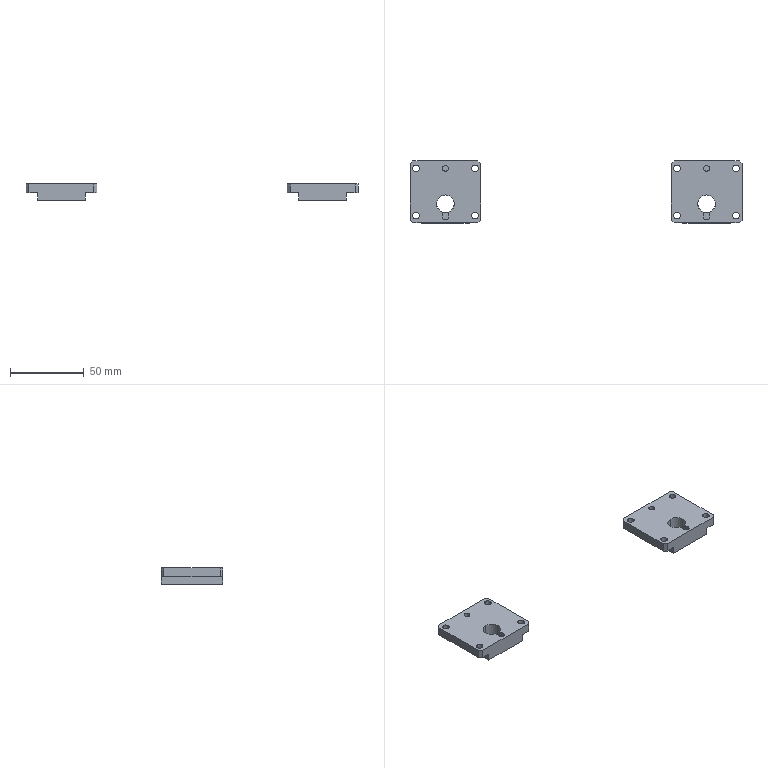NC program | NX | posted with a generic post | part box 225 x 42 x 11 mm
Whole program:
N10 G17 G21 G94 G90
(FLOOR_WALL_COPY , TOOL : D63)
N12 T01 M6
N14 G54
N16 G17 G0 G90 X-58.5 Y0. S6500 M3
N18 G43 Z30. H1
N20 Z3.
N22 G94 G1 Z0. F1500.
N24 X-55.5
N26 X55.5
N28 X58.5
N30 Z3.
N32 G0 Z30.
N34 M5
(DRILLING_COPY_1 , TOOL : D6A45)
N36 T07 M6
N38 G54
N40 G17 G0 G90 X12. Y10. S5000 M3
N42 G43 Z30. H7
N44 G94 G81 G98 Z-1. F250. R3.
N46 X5. Y16.
N48 X-5.
N50 X-12. Y10.
N52 G80
N54 G0 X-12. Y10. Z30.
N56 M5
(DRILLING_COPY_COPY , TOOL : 2.5ZT)
N58 T12 M6
N60 G54
N62 G17 G0 G90 X-12. Y10. S2000 M3
N64 G43 Z30. H12
N66 G94 G83 G98 Z-6.751 F120. Q2. R3.
N68 X-5. Y16. Z-8.251
N70 X5.
N72 X12. Y10. Z-6.751
N74 G80
N76 G0 X12. Y10. Z30.
N78 M5
(FLOOR_WALL_1 , TOOL : D10)
N80 T10 M6
N82 G54
N84 G17 G0 G90 X-31. Y-4.619 S9500 M3
N86 G43 Z30. H10
N88 Z-0.288
N90 G94 G1 X-24.5 Y-0.866 F1000.
N92 G3 X-24. Y0. R1.
N94 G1 Y19. F2500.
N96 X-22. Y21.
N98 X-21.1
N100 Y-21.
N102 X-22.
N104 X-24. Y-19.
N106 Y0.
N108 G3 X-24.5 Y0.866 R1.
N110 G1 X-31. Y4.619
N112 G0 Y-4.619 Z-0.576
N114 G1 X-24.5 Y-0.866 F1000.
N116 G3 X-24. Y0. R1.
N118 G1 Y19. F2500.
N120 X-22. Y21.
N122 X-21.1
N124 Y-21.
N126 X-22.
N128 X-24. Y-19.
N130 Y0.
N132 G3 X-24.5 Y0.866 R1.
N134 G1 X-31. Y4.619
N136 G0 Y-4.619 Z-0.865
N138 G1 X-24.5 Y-0.866 F1000.
N140 G3 X-24. Y0. R1.
N142 G1 Y19. F2500.
N144 X-22. Y21.
N146 X-21.1
N148 Y-21.
N150 X-22.
N152 X-24. Y-19.
N154 Y0.
N156 G3 X-24.5 Y0.866 R1.
N158 G1 X-31. Y4.619
N160 G0 Y-4.619 Z-1.153
N162 G1 X-24.5 Y-0.866 F1000.
N164 G3 X-24. Y0. R1.
N166 G1 Y19. F2500.
N168 X-22. Y21.
N170 X-21.1
N172 Y-21.
N174 X-22.
N176 X-24. Y-19.
N178 Y0.
N180 G3 X-24.5 Y0.866 R1.
N182 G1 X-31. Y4.619
N184 G0 Y-4.619 Z-1.441
N186 G1 X-24.5 Y-0.866 F1000.
N188 G3 X-24. Y0. R1.
N190 G1 Y19. F2500.
N192 X-22. Y21.
N194 X-21.1
N196 Y-21.
N198 X-22.
N200 X-24. Y-19.
N202 Y0.
N204 G3 X-24.5 Y0.866 R1.
N206 G1 X-31. Y4.619
N208 G0 Y-4.619 Z-1.729
N210 G1 X-24.5 Y-0.866 F1000.
N212 G3 X-24. Y0. R1.
N214 G1 Y19. F2500.
N216 X-22. Y21.
N218 X-21.1
N220 Y-21.
N222 X-22.
N224 X-24. Y-19.
N226 Y0.
N228 G3 X-24.5 Y0.866 R1.
N230 G1 X-31. Y4.619
N232 G0 Y-4.619 Z-2.018
N234 G1 X-24.5 Y-0.866 F1000.
N236 G3 X-24. Y0. R1.
N238 G1 Y19. F2500.
N240 X-22. Y21.
N242 X-21.1
N244 Y-21.
N246 X-22.
N248 X-24. Y-19.
N250 Y0.
N252 G3 X-24.5 Y0.866 R1.
N254 G1 X-31. Y4.619
N256 G0 Y-4.619 Z-2.306
N258 G1 X-24.5 Y-0.866 F1000.
N260 G3 X-24. Y0. R1.
N262 G1 Y19. F2500.
N264 X-22. Y21.
N266 X-21.1
N268 Y-21.
N270 X-22.
N272 X-24. Y-19.
N274 Y0.
N276 G3 X-24.5 Y0.866 R1.
N278 G1 X-31. Y4.619
N280 G0 Y-4.619 Z-2.594
N282 G1 X-24.5 Y-0.866 F1000.
N284 G3 X-24. Y0. R1.
N286 G1 Y19. F2500.
N288 X-22. Y21.
N290 X-21.1
N292 Y-21.
N294 X-22.
N296 X-24. Y-19.
N298 Y0.
N300 G3 X-24.5 Y0.866 R1.
N302 G1 X-31. Y4.619
N304 G0 Y-4.619 Z-2.882
N306 G1 X-24.5 Y-0.866 F1000.
N308 G3 X-24. Y0. R1.
N310 G1 Y19. F2500.
N312 X-22. Y21.
N314 X-21.1
N316 Y-21.
N318 X-22.
N320 X-24. Y-19.
N322 Y0.
N324 G3 X-24.5 Y0.866 R1.
N326 G1 X-31. Y4.619
N328 G0 Y-4.619 Z-3.171
N330 G1 X-24.5 Y-0.866 F1000.
N332 G3 X-24. Y0. R1.
N334 G1 Y19. F2500.
N336 X-22. Y21.
N338 X-21.1
N340 Y-21.
N342 X-22.
N344 X-24. Y-19.
N346 Y0.
N348 G3 X-24.5 Y0.866 R1.
N350 G1 X-31. Y4.619
N352 G0 Y-4.619 Z-3.459
N354 G1 X-24.5 Y-0.866 F1000.
N356 G3 X-24. Y0. R1.
N358 G1 Y19. F2500.
N360 X-22. Y21.
N362 X-21.1
N364 Y-21.
N366 X-22.
N368 X-24. Y-19.
N370 Y0.
N372 G3 X-24.5 Y0.866 R1.
N374 G1 X-31. Y4.619
N376 G0 Y-4.619 Z-3.747
N378 G1 X-24.5 Y-0.866 F1000.
N380 G3 X-24. Y0. R1.
N382 G1 Y19. F2500.
N384 X-22. Y21.
N386 X-21.1
N388 Y-21.
N390 X-22.
N392 X-24. Y-19.
N394 Y0.
N396 G3 X-24.5 Y0.866 R1.
N398 G1 X-31. Y4.619
N400 G0 Y-4.619 Z-4.035
N402 G1 X-24.5 Y-0.866 F1000.
N404 G3 X-24. Y0. R1.
N406 G1 Y19. F2500.
N408 X-22. Y21.
N410 X-21.1
N412 Y-21.
N414 X-22.
N416 X-24. Y-19.
N418 Y0.
N420 G3 X-24.5 Y0.866 R1.
N422 G1 X-31. Y4.619
N424 G0 Y-4.619 Z-4.324
N426 G1 X-24.5 Y-0.866 F1000.
N428 G3 X-24. Y0. R1.
N430 G1 Y19. F2500.
N432 X-22. Y21.
N434 X-21.1
N436 Y-21.
N438 X-22.
N440 X-24. Y-19.
N442 Y0.
N444 G3 X-24.5 Y0.866 R1.
N446 G1 X-31. Y4.619
N448 G0 Y-4.619 Z-4.612
N450 G1 X-24.5 Y-0.866 F1000.
N452 G3 X-24. Y0. R1.
N454 G1 Y19. F2500.
N456 X-22. Y21.
N458 X-21.1
N460 Y-21.
N462 X-22.
N464 X-24. Y-19.
N466 Y0.
N468 G3 X-24.5 Y0.866 R1.
N470 G1 X-31. Y4.619
N472 G0 Y-4.619 Z-4.9
N474 G1 X-24.5 Y-0.866 F1000.
N476 G3 X-24. Y0. R1.
N478 G1 Y19. F2500.
N480 X-22. Y21.
N482 X-21.1
N484 Y-21.
N486 X-22.
N488 X-24. Y-19.
N490 Y0.
N492 G3 X-24.5 Y0.866 R1.
N494 G1 X-31. Y4.619
N496 G0 Z30.
N498 X31.
N500 Z-0.288
N502 G1 X24.5 Y0.866 F1000.
N504 G3 X24. Y0. R1.
N506 G1 Y-19. F2500.
N508 X22. Y-21.
N510 X21.1
N512 Y21.
N514 X22.
N516 X24. Y19.
N518 Y0.
N520 G3 X24.5 Y-0.866 R1.
N522 G1 X31. Y-4.619
N524 G0 Y4.619 Z-0.576
N526 G1 X24.5 Y0.866 F1000.
N528 G3 X24. Y0. R1.
N530 G1 Y-19. F2500.
N532 X22. Y-21.
N534 X21.1
N536 Y21.
N538 X22.
N540 X24. Y19.
N542 Y0.
N544 G3 X24.5 Y-0.866 R1.
N546 G1 X31. Y-4.619
N548 G0 Y4.619 Z-0.865
N550 G1 X24.5 Y0.866 F1000.
N552 G3 X24. Y0. R1.
N554 G1 Y-19. F2500.
N556 X22. Y-21.
N558 X21.1
N560 Y21.
N562 X22.
N564 X24. Y19.
N566 Y0.
N568 G3 X24.5 Y-0.866 R1.
N570 G1 X31. Y-4.619
N572 G0 Y4.619 Z-1.153
N574 G1 X24.5 Y0.866 F1000.
N576 G3 X24. Y0. R1.
N578 G1 Y-19. F2500.
N580 X22. Y-21.
N582 X21.1
N584 Y21.
N586 X22.
N588 X24. Y19.
N590 Y0.
N592 G3 X24.5 Y-0.866 R1.
N594 G1 X31. Y-4.619
N596 G0 Y4.619 Z-1.441
N598 G1 X24.5 Y0.866 F1000.
N600 G3 X24. Y0. R1.
N602 G1 Y-19. F2500.
N604 X22. Y-21.
N606 X21.1
N608 Y21.
N610 X22.
N612 X24. Y19.
N614 Y0.
N616 G3 X24.5 Y-0.866 R1.
N618 G1 X31. Y-4.619
N620 G0 Y4.619 Z-1.729
N622 G1 X24.5 Y0.866 F1000.
N624 G3 X24. Y0. R1.
N626 G1 Y-19. F2500.
N628 X22. Y-21.
N630 X21.1
N632 Y21.
N634 X22.
N636 X24. Y19.
N638 Y0.
N640 G3 X24.5 Y-0.866 R1.
N642 G1 X31. Y-4.619
N644 G0 Y4.619 Z-2.018
N646 G1 X24.5 Y0.866 F1000.
N648 G3 X24. Y0. R1.
N650 G1 Y-19. F2500.
N652 X22. Y-21.
N654 X21.1
N656 Y21.
N658 X22.
N660 X24. Y19.
N662 Y0.
N664 G3 X24.5 Y-0.866 R1.
N666 G1 X31. Y-4.619
N668 G0 Y4.619 Z-2.306
N670 G1 X24.5 Y0.866 F1000.
N672 G3 X24. Y0. R1.
N674 G1 Y-19. F2500.
N676 X22. Y-21.
N678 X21.1
N680 Y21.
N682 X22.
N684 X24. Y19.
N686 Y0.
N688 G3 X24.5 Y-0.866 R1.
N690 G1 X31. Y-4.619
N692 G0 Y4.619 Z-2.594
N694 G1 X24.5 Y0.866 F1000.
N696 G3 X24. Y0. R1.
N698 G1 Y-19. F2500.
N700 X22. Y-21.
N702 X21.1
N704 Y21.
N706 X22.
N708 X24. Y19.
N710 Y0.
N712 G3 X24.5 Y-0.866 R1.
N714 G1 X31. Y-4.619
N716 G0 Y4.619 Z-2.882
N718 G1 X24.5 Y0.866 F1000.
N720 G3 X24. Y0. R1.
N722 G1 Y-19. F2500.
N724 X22. Y-21.
N726 X21.1
N728 Y21.
N730 X22.
N732 X24. Y19.
N734 Y0.
N736 G3 X24.5 Y-0.866 R1.
N738 G1 X31. Y-4.619
N740 G0 Y4.619 Z-3.171
N742 G1 X24.5 Y0.866 F1000.
N744 G3 X24. Y0. R1.
N746 G1 Y-19. F2500.
N748 X22. Y-21.
N750 X21.1
N752 Y21.
N754 X22.
N756 X24. Y19.
N758 Y0.
N760 G3 X24.5 Y-0.866 R1.
N762 G1 X31. Y-4.619
N764 G0 Y4.619 Z-3.459
N766 G1 X24.5 Y0.866 F1000.
N768 G3 X24. Y0. R1.
N770 G1 Y-19. F2500.
N772 X22. Y-21.
N774 X21.1
N776 Y21.
N778 X22.
N780 X24. Y19.
N782 Y0.
N784 G3 X24.5 Y-0.866 R1.
N786 G1 X31. Y-4.619
N788 G0 Y4.619 Z-3.747
N790 G1 X24.5 Y0.866 F1000.
N792 G3 X24. Y0. R1.
N794 G1 Y-19. F2500.
N796 X22. Y-21.
N798 X21.1
N800 Y21.
N802 X22.
N804 X24. Y19.
N806 Y0.
N808 G3 X24.5 Y-0.866 R1.
N810 G1 X31. Y-4.619
N812 G0 Y4.619 Z-4.035
N814 G1 X24.5 Y0.866 F1000.
N816 G3 X24. Y0. R1.
N818 G1 Y-19. F2500.
N820 X22. Y-21.
N822 X21.1
N824 Y21.
N826 X22.
N828 X24. Y19.
N830 Y0.
N832 G3 X24.5 Y-0.866 R1.
N834 G1 X31. Y-4.619
N836 G0 Y4.619 Z-4.324
N838 G1 X24.5 Y0.866 F1000.
N840 G3 X24. Y0. R1.
N842 G1 Y-19. F2500.
N844 X22. Y-21.
N846 X21.1
N848 Y21.
N850 X22.
N852 X24. Y19.
N854 Y0.
N856 G3 X24.5 Y-0.866 R1.
N858 G1 X31. Y-4.619
N860 G0 Y4.619 Z-4.612
N862 G1 X24.5 Y0.866 F1000.
N864 G3 X24. Y0. R1.
N866 G1 Y-19. F2500.
N868 X22. Y-21.
N870 X21.1
N872 Y21.
N874 X22.
N876 X24. Y19.
N878 Y0.
N880 G3 X24.5 Y-0.866 R1.
N882 G1 X31. Y-4.619
N884 G0 Y4.619 Z-4.9
N886 G1 X24.5 Y0.866 F1000.
N888 G3 X24. Y0. R1.
N890 G1 Y-19. F2500.
N892 X22. Y-21.
N894 X21.1
N896 Y21.
N898 X22.
N900 X24. Y19.
N902 Y0.
N904 G3 X24.5 Y-0.866 R1.
N906 G1 X31. Y-4.619
N908 G0 Z30.
N910 M5
(FLOOR_WALL_1_COPY , TOOL : D10JING)
N912 T11 M6
N914 G54
N916 G17 G0 G90 X-25.472 Y-27.428 S9500 M3
N918 G43 Z30. H11
N920 Z-5.
N922 G94 G1 X-24.499 Y-26.866 F1000.
N924 G3 X-23.999 Y-26. R1.
N926 G1 Y26. F1200.
N928 X-21.5
N930 Y-26.
N932 G2 X-22. Y-26.866 R1.
N934 G1 X-23.964 Y-28.
N936 X-23.464
N938 X-21.5 Y-26.866 F1000.
N940 G3 X-21. Y-26. R1.
N942 G1 Y26. F1200.
N944 G3 X-21.5 Y26.866 R1.
N946 G1 X-23.464 Y28.
N948 G0 Z30.
N950 X25.472 Y27.428
N952 Z-5.
N954 G1 X24.499 Y26.866 F1000.
N956 G3 X23.999 Y26. R1.
N958 G1 Y-26. F1200.
N960 X21.5
N962 Y26.
N964 G2 X22. Y26.866 R1.
N966 G1 X23.964 Y28.
N968 X23.464
N970 X21.5 Y26.866 F1000.
N972 G3 X21. Y26. R1.
N974 G1 Y-26. F1200.
N976 G3 X21.5 Y-26.866 R1.
N978 G1 X23.464 Y-28.
N980 G0 Z30.
N982 M5
(HOLE_MILLING_1_COPY , TOOL : D3)
N984 T03 M6
N986 G54
N988 G17 G0 G90 X-12. Y10. S9500 M3
N990 G43 Z30. H3
N992 Z0.5
N994 G94 G3 X-12.2 Y10.2 R0.2 F1250.
N996 X-12.4 Y10. R0.2
N998 X-12.4 Y10. Z0.35 I0.4 J0.
N1000 X-12.4 Y10. Z0.2 I0.4 J0.
N1002 X-12.4 Y10. Z0.05 I0.4 J0.
N1004 X-12.4 Y10. Z-0.1 I0.4 J0.
N1006 X-12.4 Y10. Z-0.25 I0.4 J0.
N1008 X-12.4 Y10. Z-0.4 I0.4 J0.
N1010 X-12.4 Y10. Z-0.55 I0.4 J0.
N1012 X-12.4 Y10. Z-0.7 I0.4 J0.
N1014 X-12.4 Y10. Z-0.85 I0.4 J0.
N1016 X-12.4 Y10. Z-1. I0.4 J0.
N1018 X-12.4 Y10. Z-1.15 I0.4 J0.
N1020 X-12.4 Y10. Z-1.3 I0.4 J0.
N1022 X-12.4 Y10. Z-1.45 I0.4 J0.
N1024 X-12.4 Y10. Z-1.6 I0.4 J0.
N1026 X-12.4 Y10. Z-1.75 I0.4 J0.
N1028 X-12.4 Y10. Z-1.9 I0.4 J0.
N1030 X-12.4 Y10. Z-2.05 I0.4 J0.
N1032 X-12.4 Y10. Z-2.2 I0.4 J0.
N1034 X-12.4 Y10. Z-2.35 I0.4 J0.
N1036 X-12.4 Y10. Z-2.5 I0.4 J0.
N1038 X-12.4 Y10. Z-2.65 I0.4 J0.
N1040 X-12.4 Y10. Z-2.8 I0.4 J0.
N1042 X-12.4 Y10. Z-2.95 I0.4 J0.
N1044 X-12.4 Y10. Z-3.1 I0.4 J0.
N1046 X-12.4 Y10. Z-3.25 I0.4 J0.
N1048 X-12.4 Y10. Z-3.4 I0.4 J0.
N1050 X-12.4 Y10. Z-3.55 I0.4 J0.
N1052 X-12.4 Y10. Z-3.7 I0.4 J0.
N1054 X-12.4 Y10. Z-3.85 I0.4 J0.
N1056 X-12.4 Y10. Z-4. I0.4 J0.
N1058 X-12.4 Y10. Z-4.15 I0.4 J0.
N1060 X-12.4 Y10. Z-4.3 I0.4 J0.
N1062 X-12.4 Y10. Z-4.45 I0.4 J0.
N1064 X-12.4 Y10. Z-4.6 I0.4 J0.
N1066 X-12.4 Y10. Z-4.75 I0.4 J0.
N1068 X-12.4 Y10. Z-4.9 I0.4 J0.
N1070 X-12.4 Y10. Z-5.05 I0.4 J0.
N1072 X-12.4 Y10. Z-5.2 I0.4 J0.
N1074 X-12.4 Y10. Z-5.35 I0.4 J0.
N1076 X-12.4 Y10. Z-5.5 I0.4 J0.
N1078 X-12.4 Y10. Z-5.65 I0.4 J0.
N1080 X-12.4 Y10. Z-5.8 I0.4 J0.
N1082 X-12.4 Y10. Z-5.95 I0.4 J0.
N1084 X-11.8 Y9.654 Z-6. R0.4
N1086 X-11.654 Y10.2 R0.4
N1088 X-11.8 Y9.654 R-0.4
N1090 X-11.727 Y9.927 R0.2
N1092 X-12. Y10. R0.2
N1094 G0 Z30.
N1096 X12.
N1098 Z0.5
N1100 G3 X11.8 Y10.2 R0.2
N1102 X11.6 Y10. R0.2
N1104 X11.6 Y10. Z0.35 I0.4 J0.
N1106 X11.6 Y10. Z0.2 I0.4 J0.
N1108 X11.6 Y10. Z0.05 I0.4 J0.
N1110 X11.6 Y10. Z-0.1 I0.4 J0.
N1112 X11.6 Y10. Z-0.25 I0.4 J0.
N1114 X11.6 Y10. Z-0.4 I0.4 J0.
N1116 X11.6 Y10. Z-0.55 I0.4 J0.
N1118 X11.6 Y10. Z-0.7 I0.4 J0.
N1120 X11.6 Y10. Z-0.85 I0.4 J0.
N1122 X11.6 Y10. Z-1. I0.4 J0.
N1124 X11.6 Y10. Z-1.15 I0.4 J0.
N1126 X11.6 Y10. Z-1.3 I0.4 J0.
N1128 X11.6 Y10. Z-1.45 I0.4 J0.
N1130 X11.6 Y10. Z-1.6 I0.4 J0.
N1132 X11.6 Y10. Z-1.75 I0.4 J0.
N1134 X11.6 Y10. Z-1.9 I0.4 J0.
N1136 X11.6 Y10. Z-2.05 I0.4 J0.
N1138 X11.6 Y10. Z-2.2 I0.4 J0.
N1140 X11.6 Y10. Z-2.35 I0.4 J0.
N1142 X11.6 Y10. Z-2.5 I0.4 J0.
N1144 X11.6 Y10. Z-2.65 I0.4 J0.
N1146 X11.6 Y10. Z-2.8 I0.4 J0.
N1148 X11.6 Y10. Z-2.95 I0.4 J0.
N1150 X11.6 Y10. Z-3.1 I0.4 J0.
N1152 X11.6 Y10. Z-3.25 I0.4 J0.
N1154 X11.6 Y10. Z-3.4 I0.4 J0.
N1156 X11.6 Y10. Z-3.55 I0.4 J0.
N1158 X11.6 Y10. Z-3.7 I0.4 J0.
N1160 X11.6 Y10. Z-3.85 I0.4 J0.
N1162 X11.6 Y10. Z-4. I0.4 J0.
N1164 X11.6 Y10. Z-4.15 I0.4 J0.
N1166 X11.6 Y10. Z-4.3 I0.4 J0.
N1168 X11.6 Y10. Z-4.45 I0.4 J0.
N1170 X11.6 Y10. Z-4.6 I0.4 J0.
N1172 X11.6 Y10. Z-4.75 I0.4 J0.
N1174 X11.6 Y10. Z-4.9 I0.4 J0.
N1176 X11.6 Y10. Z-5.05 I0.4 J0.
N1178 X11.6 Y10. Z-5.2 I0.4 J0.
N1180 X11.6 Y10. Z-5.35 I0.4 J0.
N1182 X11.6 Y10. Z-5.5 I0.4 J0.
N1184 X11.6 Y10. Z-5.65 I0.4 J0.
N1186 X11.6 Y10. Z-5.8 I0.4 J0.
N1188 X11.6 Y10. Z-5.95 I0.4 J0.
N1190 X12.2 Y9.654 Z-6. R0.4
N1192 X12.346 Y10.2 R0.4
N1194 X12.2 Y9.654 R-0.4
N1196 X12.273 Y9.927 R0.2
N1198 X12. Y10. R0.2
N1200 G0 Z30.
N1202 M5
(PLANAR_MILL_COPY_1_COPY_COPY , TOOL : D6A45)
N1204 T07 M6
N1206 G54
N1208 G17 G0 G90 X19.76 Y17.35 S9500 M3
N1210 G43 Z30. H7
N1212 Z-4.5
N1214 G94 G1 X19.741 Z-4.505 F1250.
N1216 X19.5 Y17.254 Z-4.575
N1218 X19.741 Y17.35 Z-4.644
N1220 X20.286 Z-4.79
N1222 X20.976 Y16.976 Z-5.
N1224 X21.35 Y16.286 Z-5.211
N1226 Y15.714 Z-5.364
N1228 X20.976 Y15.024 Z-5.574
N1230 X20.286 Y14.65 Z-5.784
N1232 X19.741 Z-5.931
N1234 X19.5 Y14.746 Z-6.
N1236 G3 X19.5 Y17.254 R-1.35
N1238 X20. Y16.388 R1.
N1240 G1 Z-4.5
N1242 G0 Z30.
N1244 X19.76 Y-14.65
N1246 Z-4.5
N1248 G1 X19.741 Z-4.505
N1250 X19.5 Y-14.746 Z-4.575
N1252 X19.741 Y-14.65 Z-4.644
N1254 X20.286 Z-4.79
N1256 X20.976 Y-15.024 Z-5.
N1258 X21.35 Y-15.714 Z-5.211
N1260 Y-16.286 Z-5.364
N1262 X20.976 Y-16.976 Z-5.574
N1264 X20.286 Y-17.35 Z-5.784
N1266 X19.741 Z-5.931
N1268 X19.5 Y-17.254 Z-6.
N1270 G3 X19.5 Y-14.746 R-1.35
N1272 X20. Y-15.612 R1.
N1274 G1 Z-4.5
N1276 G0 Z30.
N1278 X20.092 Y23.313
N1280 Z-4.5
N1282 G1 Z-6.
N1284 X19.643 Y22.865
N1286 G3 X19.382 Y21.9 R1.
N1288 G1 X21.959
N1290 G2 X22.666 Y21.607 R1.
N1292 G1 X24.607 Y19.666
N1294 G2 X24.9 Y18.959 R1.
N1296 G1 Y-18.959
N1298 G2 X24.607 Y-19.666 R1.
N1300 G1 X22.666 Y-21.607
N1302 G2 X21.959 Y-21.9 R1.
N1304 G1 X19.382
N1306 G3 X19.643 Y-22.865 R1.
N1308 G1 X20.092 Y-23.313
N1310 Z-4.5
N1312 G0 Z30.
N1314 X-20.092
N1316 Z-4.5
N1318 G1 Z-6.
N1320 X-19.643 Y-22.865
N1322 G3 X-19.382 Y-21.9 R1.
N1324 G1 X-21.959
N1326 G2 X-22.666 Y-21.607 R1.
N1328 G1 X-24.607 Y-19.666
N1330 G2 X-24.9 Y-18.959 R1.
N1332 G1 Y18.959
N1334 G2 X-24.607 Y19.666 R1.
N1336 G1 X-22.666 Y21.607
N1338 G2 X-21.959 Y21.9 R1.
N1340 G1 X-19.382
N1342 G3 X-19.643 Y22.865 R1.
N1344 G1 X-20.092 Y23.313
N1346 Z-4.5
N1348 G0 Z30.
N1350 X-19.76 Y-17.35
N1352 Z-4.5
N1354 G1 X-19.741 Z-4.505
N1356 X-19.5 Y-17.254 Z-4.575
N1358 X-19.741 Y-17.35 Z-4.644
N1360 X-20.286 Z-4.79
N1362 X-20.976 Y-16.976 Z-5.
N1364 X-21.35 Y-16.286 Z-5.211
N1366 Y-15.714 Z-5.364
N1368 X-20.976 Y-15.024 Z-5.574
N1370 X-20.286 Y-14.65 Z-5.784
N1372 X-19.741 Z-5.931
N1374 X-19.5 Y-14.746 Z-6.
N1376 G3 X-19.5 Y-17.254 R-1.35
N1378 X-20. Y-16.388 R1.
N1380 G1 Z-4.5
N1382 G0 Z30.
N1384 X-19.76 Y14.65
N1386 Z-4.5
N1388 G1 X-19.741 Z-4.505
N1390 X-19.5 Y14.746 Z-4.575
N1392 X-19.741 Y14.65 Z-4.644
N1394 X-20.286 Z-4.79
N1396 X-20.976 Y15.024 Z-5.
N1398 X-21.35 Y15.714 Z-5.211
N1400 Y16.286 Z-5.364
N1402 X-20.976 Y16.976 Z-5.574
N1404 X-20.286 Y17.35 Z-5.784
N1406 X-19.741 Z-5.931
N1408 X-19.5 Y17.254 Z-6.
N1410 G3 X-19.5 Y14.746 R-1.35
N1412 X-20. Y15.612 R1.
N1414 G1 Z-4.5
N1416 G0 Z30.
N1418 M5
(刀补_COPY , TOOL : D3)
N1420 T03 M6
N1422 G54
N1424 G17 G0 G90 X-12. Y10. S9500 M3
N1426 G43 Z30. H3
N1428 Z0.5
N1430 G41 G94 G1 X-12.027 Y10.096 F1250. D3
N1432 G3 X-12.45 Y10. R0.222
N1434 X-12.45 Y10. Z-1.5 I0.45 J0.
N1436 X-12.45 Y10. Z-3.5 I0.45 J0.
N1438 X-12.45 Y10. Z-5.5 I0.45 J0.
N1440 X-12. Y9.55 Z-6. R0.45
N1442 X-11.55 Y10. R0.45
N1444 X-12. Y9.55 R-0.45
N1446 X-11.904 Y9.973 R0.222
N1448 G40
N1450 G1 X-12. Y10.
N1452 G0 Z30.
N1454 X12.
N1456 Z0.5
N1458 G41 G1 X11.973 Y10.096
N1460 G3 X11.55 Y10. R0.222
N1462 X11.55 Y10. Z-1.5 I0.45 J0.
N1464 X11.55 Y10. Z-3.5 I0.45 J0.
N1466 X11.55 Y10. Z-5.5 I0.45 J0.
N1468 X12. Y9.55 Z-6. R0.45
N1470 X12.45 Y10. R0.45
N1472 X12. Y9.55 R-0.45
N1474 X12.096 Y9.973 R0.222
N1476 G40
N1478 G1 X12. Y10.
N1480 G0 Z30.
N1482 M5
N1484 M2